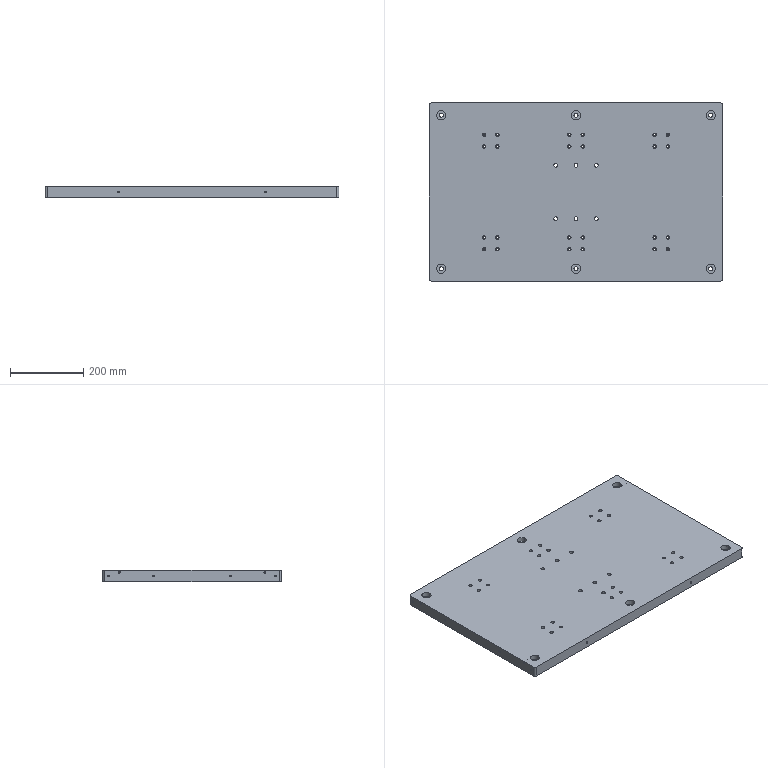NC program | Mastercam | posted with a generic post | part box 800 x 485 x 30 mm
Lines 2148 to 3510 of 3510:
N1620 T7 M6
N1630 G0 G90 G17 G54 X-367. Y-209. A0. S3000 M3
N1640 G43 H7 Z50. M8
N1650 G98 G81 Z-.7 R1. F300.
N1660 X-312. Y-167.
N1670 X-218.
N1680 Y-73.
N1690 X-312.
N1700 Y73.
N1710 X-367. Y209.
N1720 X-312. Y167.
N1730 X-218.
N1740 Y73.
N1750 X-47.
N1760 Y167.
N1770 X0. Y209.
N1780 X47. Y167.
N1790 Y73.
N1800 Y-73.
N1810 X-47.
N1820 Y-167.
N1830 X0. Y-209.
N1840 X47. Y-167.
N1850 X218. Y-73.
N1860 Y-167.
N1870 X312.
N1880 X367. Y-209.
N1890 X312. Y-73.
N1900 Y73.
N1910 X218.
N1920 Y167.
N1930 X312.
N1940 X367. Y209.
N1950 G80
N1960 M5
N1970 G91 G0 G28 Z0. M9
N1980 A0.
N1990 M01
N2000 T1 M6
N2010 G0 G90 G17 G54 X-367. Y-209. A0. S800 M3
N2020 G43 H1 Z50. M8
N2030 G98 G83 Z-24.8 R1. Q2. F100.
N2040 X0.
N2050 X367.
N2060 Y209.
N2070 X0.
N2080 X-367.
N2090 G80
N2100 M5
N2110 G91 G0 G28 Z0. M9
N2120 A0.
N2130 M01
N2140 T14 M6
N2150 G0 G90 G17 G54 X-312. Y-167. A0. S800 M3
N2160 G43 H14 Z50. M8
N2170 G98 G83 Z-24.8 R1. Q2. F100.
N2180 X-218.
N2190 Y-73.
N2200 X-312.
N2210 Y73.
N2220 Y167.
N2230 X-218.
N2240 Y73.
N2250 X-47.
N2260 Y167.
N2270 X47.
N2280 Y73.
N2290 Y-73.
N2300 X-47.
N2310 Y-167.
N2320 X47.
N2330 X218.
N2340 X312.
N2350 Y-73.
N2360 X218.
N2370 Y73.
N2380 Y167.
N2390 X312.
N2400 Y73.
N2410 G80
N2420 M5
N2430 G91 G0 G28 Z0. M9
N2440 A0.
N2450 M01
N2460 T9 M6
N2470 G0 G90 G17 G54 X-361.55 Y208. A0. S6500 M3
N2480 G43 H9 Z50. M8
N2490 Z1.2
N2500 G1 Z.2 F600.
N2510 X-360.55 F3500.
N2520 G3 X-359.55 Y209. I0. J1.
N2530 X-367. Y216.45 Z-.05 I-7.45 J0.
N2540 X-374.45 Y209. Z-.3 I0. J-7.45
N2550 X-367. Y201.55 Z-.55 I7.45 J0.
N2560 X-359.55 Y209. Z-.8 I0. J7.45
N2570 X-367. Y216.45 Z-1.05 I-7.45 J0.
N2580 X-374.45 Y209. Z-1.3 I0. J-7.45
N2590 X-367. Y201.55 Z-1.55 I7.45 J0.
N2600 X-359.55 Y209. Z-1.8 I0. J7.45
N2610 X-367. Y216.45 Z-2.05 I-7.45 J0.
N2620 X-374.45 Y209. Z-2.3 I0. J-7.45
N2630 X-367. Y201.55 Z-2.55 I7.45 J0.
N2640 X-359.55 Y209. Z-2.8 I0. J7.45
N2650 X-367. Y216.45 Z-3.05 I-7.45 J0.
N2660 X-374.45 Y209. Z-3.3 I0. J-7.45
N2670 X-367. Y201.55 Z-3.55 I7.45 J0.
N2680 X-359.55 Y209. Z-3.8 I0. J7.45
N2690 X-367. Y216.45 Z-4.05 I-7.45 J0.
N2700 X-374.45 Y209. Z-4.3 I0. J-7.45
N2710 X-367. Y201.55 Z-4.55 I7.45 J0.
N2720 X-359.55 Y209. Z-4.8 I0. J7.45
N2730 X-367. Y216.45 Z-5.05 I-7.45 J0.
N2740 X-374.45 Y209. Z-5.3 I0. J-7.45
N2750 X-367. Y201.55 Z-5.55 I7.45 J0.
N2760 X-359.55 Y209. Z-5.8 I0. J7.45
N2770 X-367. Y216.45 Z-6.05 I-7.45 J0.
N2780 X-374.45 Y209. Z-6.3 I0. J-7.45
N2790 X-367. Y201.55 Z-6.55 I7.45 J0.
N2800 X-359.55 Y209. Z-6.8 I0. J7.45
N2810 X-367. Y216.45 Z-7.05 I-7.45 J0.
N2820 X-374.45 Y209. Z-7.3 I0. J-7.45
N2830 X-367. Y201.55 Z-7.55 I7.45 J0.
N2840 X-359.55 Y209. Z-7.8 I0. J7.45
N2850 X-367. Y216.45 Z-8.05 I-7.45 J0.
N2860 X-374.45 Y209. Z-8.3 I0. J-7.45
N2870 X-367. Y201.55 Z-8.55 I7.45 J0.
N2880 X-359.55 Y209. Z-8.8 I0. J7.45
N2890 X-367. Y216.45 Z-9.05 I-7.45 J0.
N2900 X-374.45 Y209. Z-9.3 I0. J-7.45
N2910 X-367. Y201.55 Z-9.55 I7.45 J0.
N2920 X-359.55 Y209. Z-9.8 I0. J7.45
N2930 X-367. Y216.45 Z-10.05 I-7.45 J0.
N2940 X-374.45 Y209. Z-10.3 I0. J-7.45
N2950 X-367. Y201.55 Z-10.55 I7.45 J0.
N2960 X-359.55 Y209. Z-10.8 I0. J7.45
N2970 X-367. Y216.45 Z-11.05 I-7.45 J0.
N2980 X-374.45 Y209. Z-11.3 I0. J-7.45
N2990 X-367. Y201.55 Z-11.55 I7.45 J0.
N3000 X-359.55 Y209. Z-11.8 I0. J7.45
N3010 X-367. Y216.45 Z-12.05 I-7.45 J0.
N3020 X-374.45 Y209. Z-12.3 I0. J-7.45
N3030 X-367. Y201.55 Z-12.55 I7.45 J0.
N3040 X-359.55 Y209. Z-12.8 I0. J7.45
N3050 X-362.621 Y215.027 Z-12.95 I-7.45 J0.
N3060 X-367. Y216.45 I-4.379 J-6.027
N3070 X-374.45 Y209. I0. J-7.45
N3080 X-367. Y201.55 I7.45 J0.
N3090 X-359.55 Y209. I0. J7.45
N3100 X-362.621 Y215.027 I-7.45 J0.
N3110 X-363.209 Y215.218 I-.588 J-.809
N3120 X-364.018 Y214.806 I0. J-1.
N3130 G1 X-364.606 Y213.997
N3140 G0 Z50.
N3150 X-361.55 Y-210.
N3160 Z1.2
N3170 G1 Z.2 F600.
N3180 X-360.55 F3500.
N3190 G3 X-359.55 Y-209. I0. J1.
N3200 X-367. Y-201.55 Z-.05 I-7.45 J0.
N3210 X-374.45 Y-209. Z-.3 I0. J-7.45
N3220 X-367. Y-216.45 Z-.55 I7.45 J0.
N3230 X-359.55 Y-209. Z-.8 I0. J7.45
N3240 X-367. Y-201.55 Z-1.05 I-7.45 J0.
N3250 X-374.45 Y-209. Z-1.3 I0. J-7.45
N3260 X-367. Y-216.45 Z-1.55 I7.45 J0.
N3270 X-359.55 Y-209. Z-1.8 I0. J7.45
N3280 X-367. Y-201.55 Z-2.05 I-7.45 J0.
N3290 X-374.45 Y-209. Z-2.3 I0. J-7.45
N3300 X-367. Y-216.45 Z-2.55 I7.45 J0.
N3310 X-359.55 Y-209. Z-2.8 I0. J7.45
N3320 X-367. Y-201.55 Z-3.05 I-7.45 J0.
N3330 X-374.45 Y-209. Z-3.3 I0. J-7.45
N3340 X-367. Y-216.45 Z-3.55 I7.45 J0.
N3350 X-359.55 Y-209. Z-3.8 I0. J7.45
N3360 X-367. Y-201.55 Z-4.05 I-7.45 J0.
N3370 X-374.45 Y-209. Z-4.3 I0. J-7.45
N3380 X-367. Y-216.45 Z-4.55 I7.45 J0.
N3390 X-359.55 Y-209. Z-4.8 I0. J7.45
N3400 X-367. Y-201.55 Z-5.05 I-7.45 J0.
N3410 X-374.45 Y-209. Z-5.3 I0. J-7.45
N3420 X-367. Y-216.45 Z-5.55 I7.45 J0.
N3430 X-359.55 Y-209. Z-5.8 I0. J7.45
N3440 X-367. Y-201.55 Z-6.05 I-7.45 J0.
N3450 X-374.45 Y-209. Z-6.3 I0. J-7.45
N3460 X-367. Y-216.45 Z-6.55 I7.45 J0.
N3470 X-359.55 Y-209. Z-6.8 I0. J7.45
N3480 X-367. Y-201.55 Z-7.05 I-7.45 J0.
N3490 X-374.45 Y-209. Z-7.3 I0. J-7.45
N3500 X-367. Y-216.45 Z-7.55 I7.45 J0.
N3510 X-359.55 Y-209. Z-7.8 I0. J7.45
N3520 X-367. Y-201.55 Z-8.05 I-7.45 J0.
N3530 X-374.45 Y-209. Z-8.3 I0. J-7.45
N3540 X-367. Y-216.45 Z-8.55 I7.45 J0.
N3550 X-359.55 Y-209. Z-8.8 I0. J7.45
N3560 X-367. Y-201.55 Z-9.05 I-7.45 J0.
N3570 X-374.45 Y-209. Z-9.3 I0. J-7.45
N3580 X-367. Y-216.45 Z-9.55 I7.45 J0.
N3590 X-359.55 Y-209. Z-9.8 I0. J7.45
N3600 X-367. Y-201.55 Z-10.05 I-7.45 J0.
N3610 X-374.45 Y-209. Z-10.3 I0. J-7.45
N3620 X-367. Y-216.45 Z-10.55 I7.45 J0.
N3630 X-359.55 Y-209. Z-10.8 I0. J7.45
N3640 X-367. Y-201.55 Z-11.05 I-7.45 J0.
N3650 X-374.45 Y-209. Z-11.3 I0. J-7.45
N3660 X-367. Y-216.45 Z-11.55 I7.45 J0.
N3670 X-359.55 Y-209. Z-11.8 I0. J7.45
N3680 X-367. Y-201.55 Z-12.05 I-7.45 J0.
N3690 X-374.45 Y-209. Z-12.3 I0. J-7.45
N3700 X-367. Y-216.45 Z-12.55 I7.45 J0.
N3710 X-359.55 Y-209. Z-12.8 I0. J7.45
N3720 X-362.621 Y-202.973 Z-12.95 I-7.45 J0.
N3730 X-367. Y-201.55 I-4.379 J-6.027
N3740 X-374.45 Y-209. I0. J-7.45
N3750 X-367. Y-216.45 I7.45 J0.
N3760 X-359.55 Y-209. I0. J7.45
N3770 X-362.621 Y-202.973 I-7.45 J0.
N3780 X-363.209 Y-202.782 I-.588 J-.809
N3790 X-364.018 Y-203.194 I0. J-1.
N3800 G1 X-364.606 Y-204.003
N3810 G0 Z50.
N3820 X5.45 Y-210.
N3830 Z1.2
N3840 G1 Z.2 F600.
N3850 X6.45 F3500.
N3860 G3 X7.45 Y-209. I0. J1.
N3870 X0. Y-201.55 Z-.05 I-7.45 J0.
N3880 X-7.45 Y-209. Z-.3 I0. J-7.45
N3890 X0. Y-216.45 Z-.55 I7.45 J0.
N3900 X7.45 Y-209. Z-.8 I0. J7.45
N3910 X0. Y-201.55 Z-1.05 I-7.45 J0.
N3920 X-7.45 Y-209. Z-1.3 I0. J-7.45
N3930 X0. Y-216.45 Z-1.55 I7.45 J0.
N3940 X7.45 Y-209. Z-1.8 I0. J7.45
N3950 X0. Y-201.55 Z-2.05 I-7.45 J0.
N3960 X-7.45 Y-209. Z-2.3 I0. J-7.45
N3970 X0. Y-216.45 Z-2.55 I7.45 J0.
N3980 X7.45 Y-209. Z-2.8 I0. J7.45
N3990 X0. Y-201.55 Z-3.05 I-7.45 J0.
N4000 X-7.45 Y-209. Z-3.3 I0. J-7.45
N4010 X0. Y-216.45 Z-3.55 I7.45 J0.
N4020 X7.45 Y-209. Z-3.8 I0. J7.45
N4030 X0. Y-201.55 Z-4.05 I-7.45 J0.
N4040 X-7.45 Y-209. Z-4.3 I0. J-7.45
N4050 X0. Y-216.45 Z-4.55 I7.45 J0.
N4060 X7.45 Y-209. Z-4.8 I0. J7.45
N4070 X0. Y-201.55 Z-5.05 I-7.45 J0.
N4080 X-7.45 Y-209. Z-5.3 I0. J-7.45
N4090 X0. Y-216.45 Z-5.55 I7.45 J0.
N4100 X7.45 Y-209. Z-5.8 I0. J7.45
N4110 X0. Y-201.55 Z-6.05 I-7.45 J0.
N4120 X-7.45 Y-209. Z-6.3 I0. J-7.45
N4130 X0. Y-216.45 Z-6.55 I7.45 J0.
N4140 X7.45 Y-209. Z-6.8 I0. J7.45
N4150 X0. Y-201.55 Z-7.05 I-7.45 J0.
N4160 X-7.45 Y-209. Z-7.3 I0. J-7.45
N4170 X0. Y-216.45 Z-7.55 I7.45 J0.
N4180 X7.45 Y-209. Z-7.8 I0. J7.45
N4190 X0. Y-201.55 Z-8.05 I-7.45 J0.
N4200 X-7.45 Y-209. Z-8.3 I0. J-7.45
N4210 X0. Y-216.45 Z-8.55 I7.45 J0.
N4220 X7.45 Y-209. Z-8.8 I0. J7.45
N4230 X0. Y-201.55 Z-9.05 I-7.45 J0.
N4240 X-7.45 Y-209. Z-9.3 I0. J-7.45
N4250 X0. Y-216.45 Z-9.55 I7.45 J0.
N4260 X7.45 Y-209. Z-9.8 I0. J7.45
N4270 X0. Y-201.55 Z-10.05 I-7.45 J0.
N4280 X-7.45 Y-209. Z-10.3 I0. J-7.45
N4290 X0. Y-216.45 Z-10.55 I7.45 J0.
N4300 X7.45 Y-209. Z-10.8 I0. J7.45
N4310 X0. Y-201.55 Z-11.05 I-7.45 J0.
N4320 X-7.45 Y-209. Z-11.3 I0. J-7.45
N4330 X0. Y-216.45 Z-11.55 I7.45 J0.
N4340 X7.45 Y-209. Z-11.8 I0. J7.45
N4350 X0. Y-201.55 Z-12.05 I-7.45 J0.
N4360 X-7.45 Y-209. Z-12.3 I0. J-7.45
N4370 X0. Y-216.45 Z-12.55 I7.45 J0.
N4380 X7.45 Y-209. Z-12.8 I0. J7.45
N4390 X4.379 Y-202.973 Z-12.95 I-7.45 J0.
N4400 X0. Y-201.55 I-4.379 J-6.027
N4410 X-7.45 Y-209. I0. J-7.45
N4420 X0. Y-216.45 I7.45 J0.
N4430 X7.45 Y-209. I0. J7.45
N4440 X4.379 Y-202.973 I-7.45 J0.
N4450 X3.791 Y-202.782 I-.588 J-.809
N4460 X2.982 Y-203.194 I0. J-1.
N4470 G1 X2.394 Y-204.003
N4480 G0 Z50.
N4490 X372.45 Y-210.
N4500 Z1.2
N4510 G1 Z.2 F600.
N4520 X373.45 F3500.
N4530 G3 X374.45 Y-209. I0. J1.
N4540 X367. Y-201.55 Z-.05 I-7.45 J0.
N4550 X359.55 Y-209. Z-.3 I0. J-7.45
N4560 X367. Y-216.45 Z-.55 I7.45 J0.
N4570 X374.45 Y-209. Z-.8 I0. J7.45
N4580 X367. Y-201.55 Z-1.05 I-7.45 J0.
N4590 X359.55 Y-209. Z-1.3 I0. J-7.45
N4600 X367. Y-216.45 Z-1.55 I7.45 J0.
N4610 X374.45 Y-209. Z-1.8 I0. J7.45
N4620 X367. Y-201.55 Z-2.05 I-7.45 J0.
N4630 X359.55 Y-209. Z-2.3 I0. J-7.45
N4640 X367. Y-216.45 Z-2.55 I7.45 J0.
N4650 X374.45 Y-209. Z-2.8 I0. J7.45
N4660 X367. Y-201.55 Z-3.05 I-7.45 J0.
N4670 X359.55 Y-209. Z-3.3 I0. J-7.45
N4680 X367. Y-216.45 Z-3.55 I7.45 J0.
N4690 X374.45 Y-209. Z-3.8 I0. J7.45
N4700 X367. Y-201.55 Z-4.05 I-7.45 J0.
N4710 X359.55 Y-209. Z-4.3 I0. J-7.45
N4720 X367. Y-216.45 Z-4.55 I7.45 J0.
N4730 X374.45 Y-209. Z-4.8 I0. J7.45
N4740 X367. Y-201.55 Z-5.05 I-7.45 J0.
N4750 X359.55 Y-209. Z-5.3 I0. J-7.45
N4760 X367. Y-216.45 Z-5.55 I7.45 J0.
N4770 X374.45 Y-209. Z-5.8 I0. J7.45
N4780 X367. Y-201.55 Z-6.05 I-7.45 J0.
N4790 X359.55 Y-209. Z-6.3 I0. J-7.45
N4800 X367. Y-216.45 Z-6.55 I7.45 J0.
N4810 X374.45 Y-209. Z-6.8 I0. J7.45
N4820 X367. Y-201.55 Z-7.05 I-7.45 J0.
N4830 X359.55 Y-209. Z-7.3 I0. J-7.45
N4840 X367. Y-216.45 Z-7.55 I7.45 J0.
N4850 X374.45 Y-209. Z-7.8 I0. J7.45
N4860 X367. Y-201.55 Z-8.05 I-7.45 J0.
N4870 X359.55 Y-209. Z-8.3 I0. J-7.45
N4880 X367. Y-216.45 Z-8.55 I7.45 J0.
N4890 X374.45 Y-209. Z-8.8 I0. J7.45
N4900 X367. Y-201.55 Z-9.05 I-7.45 J0.
N4910 X359.55 Y-209. Z-9.3 I0. J-7.45
N4920 X367. Y-216.45 Z-9.55 I7.45 J0.
N4930 X374.45 Y-209. Z-9.8 I0. J7.45
N4940 X367. Y-201.55 Z-10.05 I-7.45 J0.
N4950 X359.55 Y-209. Z-10.3 I0. J-7.45
N4960 X367. Y-216.45 Z-10.55 I7.45 J0.
N4970 X374.45 Y-209. Z-10.8 I0. J7.45
N4980 X367. Y-201.55 Z-11.05 I-7.45 J0.
N4990 X359.55 Y-209. Z-11.3 I0. J-7.45
N5000 X367. Y-216.45 Z-11.55 I7.45 J0.
N5010 X374.45 Y-209. Z-11.8 I0. J7.45
N5020 X367. Y-201.55 Z-12.05 I-7.45 J0.
N5030 X359.55 Y-209. Z-12.3 I0. J-7.45
N5040 X367. Y-216.45 Z-12.55 I7.45 J0.
N5050 X374.45 Y-209. Z-12.8 I0. J7.45
N5060 X371.379 Y-202.973 Z-12.95 I-7.45 J0.
N5070 X367. Y-201.55 I-4.379 J-6.027
N5080 X359.55 Y-209. I0. J-7.45
N5090 X367. Y-216.45 I7.45 J0.
N5100 X374.45 Y-209. I0. J7.45
N5110 X371.379 Y-202.973 I-7.45 J0.
N5120 X370.791 Y-202.782 I-.588 J-.809
N5130 X369.982 Y-203.194 I0. J-1.
N5140 G1 X369.394 Y-204.003
N5150 G0 Z50.
N5160 X372.45 Y208.
N5170 Z1.2
N5180 G1 Z.2 F600.
N5190 X373.45 F3500.
N5200 G3 X374.45 Y209. I0. J1.
N5210 X367. Y216.45 Z-.05 I-7.45 J0.
N5220 X359.55 Y209. Z-.3 I0. J-7.45
N5230 X367. Y201.55 Z-.55 I7.45 J0.
N5240 X374.45 Y209. Z-.8 I0. J7.45
N5250 X367. Y216.45 Z-1.05 I-7.45 J0.
N5260 X359.55 Y209. Z-1.3 I0. J-7.45
N5270 X367. Y201.55 Z-1.55 I7.45 J0.
N5280 X374.45 Y209. Z-1.8 I0. J7.45
N5290 X367. Y216.45 Z-2.05 I-7.45 J0.
N5300 X359.55 Y209. Z-2.3 I0. J-7.45
N5310 X367. Y201.55 Z-2.55 I7.45 J0.
N5320 X374.45 Y209. Z-2.8 I0. J7.45
N5330 X367. Y216.45 Z-3.05 I-7.45 J0.
N5340 X359.55 Y209. Z-3.3 I0. J-7.45
N5350 X367. Y201.55 Z-3.55 I7.45 J0.
N5360 X374.45 Y209. Z-3.8 I0. J7.45
N5370 X367. Y216.45 Z-4.05 I-7.45 J0.
N5380 X359.55 Y209. Z-4.3 I0. J-7.45
N5390 X367. Y201.55 Z-4.55 I7.45 J0.
N5400 X374.45 Y209. Z-4.8 I0. J7.45
N5410 X367. Y216.45 Z-5.05 I-7.45 J0.
N5420 X359.55 Y209. Z-5.3 I0. J-7.45
N5430 X367. Y201.55 Z-5.55 I7.45 J0.
N5440 X374.45 Y209. Z-5.8 I0. J7.45
N5450 X367. Y216.45 Z-6.05 I-7.45 J0.
N5460 X359.55 Y209. Z-6.3 I0. J-7.45
N5470 X367. Y201.55 Z-6.55 I7.45 J0.
N5480 X374.45 Y209. Z-6.8 I0. J7.45
N5490 X367. Y216.45 Z-7.05 I-7.45 J0.
N5500 X359.55 Y209. Z-7.3 I0. J-7.45
N5510 X367. Y201.55 Z-7.55 I7.45 J0.
N5520 X374.45 Y209. Z-7.8 I0. J7.45
N5530 X367. Y216.45 Z-8.05 I-7.45 J0.
N5540 X359.55 Y209. Z-8.3 I0. J-7.45
N5550 X367. Y201.55 Z-8.55 I7.45 J0.
N5560 X374.45 Y209. Z-8.8 I0. J7.45
N5570 X367. Y216.45 Z-9.05 I-7.45 J0.
N5580 X359.55 Y209. Z-9.3 I0. J-7.45
N5590 X367. Y201.55 Z-9.55 I7.45 J0.
N5600 X374.45 Y209. Z-9.8 I0. J7.45
N5610 X367. Y216.45 Z-10.05 I-7.45 J0.
N5620 X359.55 Y209. Z-10.3 I0. J-7.45
N5630 X367. Y201.55 Z-10.55 I7.45 J0.
N5640 X374.45 Y209. Z-10.8 I0. J7.45
N5650 X367. Y216.45 Z-11.05 I-7.45 J0.
N5660 X359.55 Y209. Z-11.3 I0. J-7.45
N5670 X367. Y201.55 Z-11.55 I7.45 J0.
N5680 X374.45 Y209. Z-11.8 I0. J7.45
N5690 X367. Y216.45 Z-12.05 I-7.45 J0.
N5700 X359.55 Y209. Z-12.3 I0. J-7.45
N5710 X367. Y201.55 Z-12.55 I7.45 J0.
N5720 X374.45 Y209. Z-12.8 I0. J7.45
N5730 X371.379 Y215.027 Z-12.95 I-7.45 J0.
N5740 X367. Y216.45 I-4.379 J-6.027
N5750 X359.55 Y209. I0. J-7.45
N5760 X367. Y201.55 I7.45 J0.
N5770 X374.45 Y209. I0. J7.45
N5780 X371.379 Y215.027 I-7.45 J0.
N5790 X370.791 Y215.218 I-.588 J-.809
N5800 X369.982 Y214.806 I0. J-1.
N5810 G1 X369.394 Y213.997
N5820 G0 Z50.
N5830 X5.45 Y208.
N5840 Z1.2
N5850 G1 Z.2 F600.
N5860 X6.45 F3500.
N5870 G3 X7.45 Y209. I0. J1.
N5880 X0. Y216.45 Z-.05 I-7.45 J0.
N5890 X-7.45 Y209. Z-.3 I0. J-7.45
N5900 X0. Y201.55 Z-.55 I7.45 J0.
N5910 X7.45 Y209. Z-.8 I0. J7.45
N5920 X0. Y216.45 Z-1.05 I-7.45 J0.
N5930 X-7.45 Y209. Z-1.3 I0. J-7.45
N5940 X0. Y201.55 Z-1.55 I7.45 J0.
N5950 X7.45 Y209. Z-1.8 I0. J7.45
N5960 X0. Y216.45 Z-2.05 I-7.45 J0.
N5970 X-7.45 Y209. Z-2.3 I0. J-7.45
N5980 X0. Y201.55 Z-2.55 I7.45 J0.
N5990 X7.45 Y209. Z-2.8 I0. J7.45
N6000 X0. Y216.45 Z-3.05 I-7.45 J0.
N6010 X-7.45 Y209. Z-3.3 I0. J-7.45
N6020 X0. Y201.55 Z-3.55 I7.45 J0.
N6030 X7.45 Y209. Z-3.8 I0. J7.45
N6040 X0. Y216.45 Z-4.05 I-7.45 J0.
N6050 X-7.45 Y209. Z-4.3 I0. J-7.45
N6060 X0. Y201.55 Z-4.55 I7.45 J0.
N6070 X7.45 Y209. Z-4.8 I0. J7.45
N6080 X0. Y216.45 Z-5.05 I-7.45 J0.
N6090 X-7.45 Y209. Z-5.3 I0. J-7.45
N6100 X0. Y201.55 Z-5.55 I7.45 J0.
N6110 X7.45 Y209. Z-5.8 I0. J7.45
N6120 X0. Y216.45 Z-6.05 I-7.45 J0.
N6130 X-7.45 Y209. Z-6.3 I0. J-7.45
N6140 X0. Y201.55 Z-6.55 I7.45 J0.
N6150 X7.45 Y209. Z-6.8 I0. J7.45
N6160 X0. Y216.45 Z-7.05 I-7.45 J0.
N6170 X-7.45 Y209. Z-7.3 I0. J-7.45
N6180 X0. Y201.55 Z-7.55 I7.45 J0.
N6190 X7.45 Y209. Z-7.8 I0. J7.45
N6200 X0. Y216.45 Z-8.05 I-7.45 J0.
N6210 X-7.45 Y209. Z-8.3 I0. J-7.45
N6220 X0. Y201.55 Z-8.55 I7.45 J0.
N6230 X7.45 Y209. Z-8.8 I0. J7.45
N6240 X0. Y216.45 Z-9.05 I-7.45 J0.
N6250 X-7.45 Y209. Z-9.3 I0. J-7.45
N6260 X0. Y201.55 Z-9.55 I7.45 J0.
N6270 X7.45 Y209. Z-9.8 I0. J7.45
N6280 X0. Y216.45 Z-10.05 I-7.45 J0.
N6290 X-7.45 Y209. Z-10.3 I0. J-7.45
N6300 X0. Y201.55 Z-10.55 I7.45 J0.
N6310 X7.45 Y209. Z-10.8 I0. J7.45
N6320 X0. Y216.45 Z-11.05 I-7.45 J0.
N6330 X-7.45 Y209. Z-11.3 I0. J-7.45
N6340 X0. Y201.55 Z-11.55 I7.45 J0.
N6350 X7.45 Y209. Z-11.8 I0. J7.45
N6360 X0. Y216.45 Z-12.05 I-7.45 J0.
N6370 X-7.45 Y209. Z-12.3 I0. J-7.45
N6380 X0. Y201.55 Z-12.55 I7.45 J0.
N6390 X7.45 Y209. Z-12.8 I0. J7.45
N6400 X4.379 Y215.027 Z-12.95 I-7.45 J0.
N6410 X0. Y216.45 I-4.379 J-6.027
N6420 X-7.45 Y209. I0. J-7.45
N6430 X0. Y201.55 I7.45 J0.
N6440 X7.45 Y209. I0. J7.45
N6450 X4.379 Y215.027 I-7.45 J0.
N6460 X3.791 Y215.218 I-.588 J-.809
N6470 X2.982 Y214.806 I0. J-1.
N6480 G1 X2.394 Y213.997
N6490 G0 Z50.
N6500 M5
N6510 G91 G28 Z0. M9
N6520 A0.
N6530 M01
N6540 T10 M6
N6550 G0 G90 G17 G54 X-361.47 Y208. A0. S6500 M3
N6560 G43 H10 Z50. M8
N6570 Z-12.
N6580 G1 Z-13. F600.
N6590 X-360.47 F1000.
N6600 G3 X-359.47 Y209. I0. J1.
N6610 X-367. Y216.53 I-7.53 J0.
N6620 X-374.53 Y209. I0. J-7.53
N6630 X-367. Y201.47 I7.53 J0.
N6640 X-359.47 Y209. I0. J7.53
N6650 X-360.47 Y210. I-1. J0.
N6660 G1 X-361.47
N6670 Y208.
N6680 X-360.47
N6690 G3 X-359.47 Y209. I0. J1.
N6700 X-367. Y216.53 I-7.53 J0.
N6710 X-374.53 Y209. I0. J-7.53
N6720 X-367. Y201.47 I7.53 J0.
N6730 X-359.47 Y209. I0. J7.53
N6740 X-360.47 Y210. I-1. J0.
N6750 G1 X-361.47
N6760 G0 Z50.
N6770 Y-210.
N6780 Z-12.
N6790 G1 Z-13. F600.
N6800 X-360.47 F1000.
N6810 G3 X-359.47 Y-209. I0. J1.
N6820 X-367. Y-201.47 I-7.53 J0.
N6830 X-374.53 Y-209. I0. J-7.53
N6840 X-367. Y-216.53 I7.53 J0.
N6850 X-359.47 Y-209. I0. J7.53
N6860 X-360.47 Y-208. I-1. J0.
N6870 G1 X-361.47
N6880 Y-210.
N6890 X-360.47
N6900 G3 X-359.47 Y-209. I0. J1.
N6910 X-367. Y-201.47 I-7.53 J0.
N6920 X-374.53 Y-209. I0. J-7.53
N6930 X-367. Y-216.53 I7.53 J0.
N6940 X-359.47 Y-209. I0. J7.53
N6950 X-360.47 Y-208. I-1. J0.
N6960 G1 X-361.47
N6970 G0 Z50.
N6980 X5.53 Y-210.
N6990 Z-12.
N7000 G1 Z-13. F600.
N7010 X6.53 F1000.
N7020 G3 X7.53 Y-209. I0. J1.
N7030 X0. Y-201.47 I-7.53 J0.
N7040 X-7.53 Y-209. I0. J-7.53
N7050 X0. Y-216.53 I7.53 J0.
N7060 X7.53 Y-209. I0. J7.53
N7070 X6.53 Y-208. I-1. J0.
N7080 G1 X5.53
N7090 Y-210.
N7100 X6.53
N7110 G3 X7.53 Y-209. I0. J1.
N7120 X0. Y-201.47 I-7.53 J0.
N7130 X-7.53 Y-209. I0. J-7.53
N7140 X0. Y-216.53 I7.53 J0.
N7150 X7.53 Y-209. I0. J7.53
N7160 X6.53 Y-208. I-1. J0.
N7170 G1 X5.53
N7180 G0 Z50.
N7190 X372.53 Y-210.
N7200 Z-12.
N7210 G1 Z-13. F600.
N7220 X373.53 F1000.
N7230 G3 X374.53 Y-209. I0. J1.
N7240 X367. Y-201.47 I-7.53 J0.
N7250 X359.47 Y-209. I0. J-7.53
N7260 X367. Y-216.53 I7.53 J0.
N7270 X374.53 Y-209. I0. J7.53
N7280 X373.53 Y-208. I-1. J0.
N7290 G1 X372.53
N7300 Y-210.
N7310 X373.53
N7320 G3 X374.53 Y-209. I0. J1.
N7330 X367. Y-201.47 I-7.53 J0.
N7340 X359.47 Y-209. I0. J-7.53
N7350 X367. Y-216.53 I7.53 J0.
N7360 X374.53 Y-209. I0. J7.53
N7370 X373.53 Y-208. I-1. J0.
N7380 G1 X372.53
N7390 G0 Z50.
N7400 Y208.
N7410 Z-12.
N7420 G1 Z-13. F600.
N7430 X373.53 F1000.
N7440 G3 X374.53 Y209. I0. J1.
N7450 X367. Y216.53 I-7.53 J0.
N7460 X359.47 Y209. I0. J-7.53
N7470 X367. Y201.47 I7.53 J0.
N7480 X374.53 Y209. I0. J7.53
N7490 X373.53 Y210. I-1. J0.
N7500 G1 X372.53
N7510 Y208.
N7520 X373.53
N7530 G3 X374.53 Y209. I0. J1.
N7540 X367. Y216.53 I-7.53 J0.
N7550 X359.47 Y209. I0. J-7.53
N7560 X367. Y201.47 I7.53 J0.
N7570 X374.53 Y209. I0. J7.53
N7580 X373.53 Y210. I-1. J0.
N7590 G1 X372.53
N7600 G0 Z50.
N7610 X5.53 Y208.
N7620 Z-12.
N7630 G1 Z-13. F600.
N7640 X6.53 F1000.
N7650 G3 X7.53 Y209. I0. J1.
N7660 X0. Y216.53 I-7.53 J0.
N7670 X-7.53 Y209. I0. J-7.53
N7680 X0. Y201.47 I7.53 J0.
N7690 X7.53 Y209. I0. J7.53
N7700 X6.53 Y210. I-1. J0.
N7710 G1 X5.53
N7720 Y208.
N7730 X6.53
N7740 G3 X7.53 Y209. I0. J1.
N7750 X0. Y216.53 I-7.53 J0.
N7760 X-7.53 Y209. I0. J-7.53
N7770 X0. Y201.47 I7.53 J0.
N7780 X7.53 Y209. I0. J7.53
N7790 X6.53 Y210. I-1. J0.
N7800 G1 X5.53
N7810 G0 Z50.
N7820 X-243.99 Y119.
N7830 Z1.
N7840 G1 Z-24.95 F600.
N7850 X-242.99 F1000.
N7860 G3 X-241.99 Y120. I0. J1.
N7870 X-265. Y143.01 I-23.01 J0.
N7880 X-288.01 Y120. I0. J-23.01
N7890 X-265. Y96.99 I23.01 J0.
N7900 X-241.99 Y120. I0. J23.01
N7910 X-242.99 Y121. I-1. J0.
N7920 G1 X-243.99
N7930 Y119.
N7940 X-242.99
N7950 G3 X-241.99 Y120. I0. J1.
N7960 X-265. Y143.01 I-23.01 J0.
N7970 X-288.01 Y120. I0. J-23.01
N7980 X-265. Y96.99 I23.01 J0.
N7990 X-241.99 Y120. I0. J23.01
N8000 X-242.99 Y121. I-1. J0.
N8010 G1 X-243.99
N8020 G0 Z50.
N8030 Y-121.
N8040 Z1.
N8050 G1 Z-24.95 F600.
N8060 X-242.99 F1000.
N8070 G3 X-241.99 Y-120. I0. J1.
N8080 X-265. Y-96.99 I-23.01 J0.
N8090 X-288.01 Y-120. I0. J-23.01
N8100 X-265. Y-143.01 I23.01 J0.
N8110 X-241.99 Y-120. I0. J23.01
N8120 X-242.99 Y-119. I-1. J0.
N8130 G1 X-243.99
N8140 Y-121.
N8150 X-242.99
N8160 G3 X-241.99 Y-120. I0. J1.
N8170 X-265. Y-96.99 I-23.01 J0.
N8180 X-288.01 Y-120. I0. J-23.01
N8190 X-265. Y-143.01 I23.01 J0.
N8200 X-241.99 Y-120. I0. J23.01
N8210 X-242.99 Y-119. I-1. J0.
N8220 G1 X-243.99
N8230 G0 Z50.
N8240 X21.01 Y-121.
N8250 Z1.
N8260 G1 Z-24.95 F600.
N8270 X22.01 F1000.
N8280 G3 X23.01 Y-120. I0. J1.
N8290 X0. Y-96.99 I-23.01 J0.
N8300 X-23.01 Y-120. I0. J-23.01
N8310 X0. Y-143.01 I23.01 J0.
N8320 X23.01 Y-120. I0. J23.01
N8330 X22.01 Y-119. I-1. J0.
N8340 G1 X21.01
N8350 Y-121.
N8360 X22.01
N8370 G3 X23.01 Y-120. I0. J1.
N8380 X0. Y-96.99 I-23.01 J0.
N8390 X-23.01 Y-120. I0. J-23.01
N8400 X0. Y-143.01 I23.01 J0.
N8410 X23.01 Y-120. I0. J23.01
N8420 X22.01 Y-119. I-1. J0.
N8430 G1 X21.01
N8440 G0 Z50.
N8450 Y119.
N8460 Z1.
N8470 G1 Z-24.95 F600.
N8480 X22.01 F1000.
N8490 G3 X23.01 Y120. I0. J1.
N8500 X0. Y143.01 I-23.01 J0.
N8510 X-23.01 Y120. I0. J-23.01
N8520 X0. Y96.99 I23.01 J0.
N8530 X23.01 Y120. I0. J23.01
N8540 X22.01 Y121. I-1. J0.
N8550 G1 X21.01
N8560 Y119.
N8570 X22.01
N8580 G3 X23.01 Y120. I0. J1.
N8590 X0. Y143.01 I-23.01 J0.
N8600 X-23.01 Y120. I0. J-23.01
N8610 X0. Y96.99 I23.01 J0.
N8620 X23.01 Y120. I0. J23.01
N8630 X22.01 Y121. I-1. J0.
N8640 G1 X21.01
N8650 G0 Z50.
N8660 X286.01 Y119.
N8670 Z1.
N8680 G1 Z-24.95 F600.
N8690 X287.01 F1000.
N8700 G3 X288.01 Y120. I0. J1.
N8710 X265. Y143.01 I-23.01 J0.
N8720 X241.99 Y120. I0. J-23.01
N8730 X265. Y96.99 I23.01 J0.
N8740 X288.01 Y120. I0. J23.01
N8750 X287.01 Y121. I-1. J0.
N8760 G1 X286.01
N8770 Y119.
N8780 X287.01
N8790 G3 X288.01 Y120. I0. J1.
N8800 X265. Y143.01 I-23.01 J0.
N8810 X241.99 Y120. I0. J-23.01
N8820 X265. Y96.99 I23.01 J0.
N8830 X288.01 Y120. I0. J23.01
N8840 X287.01 Y121. I-1. J0.
N8850 G1 X286.01
N8860 G0 Z50.
N8870 Y-121.
N8880 Z1.
N8890 G1 Z-24.95 F600.
N8900 X287.01 F1000.
N8910 G3 X288.01 Y-120. I0. J1.
N8920 X265. Y-96.99 I-23.01 J0.
N8930 X241.99 Y-120. I0. J-23.01
N8940 X265. Y-143.01 I23.01 J0.
N8950 X288.01 Y-120. I0. J23.01
N8960 X287.01 Y-119. I-1. J0.
N8970 G1 X286.01
N8980 Y-121.
N8990 X287.01
N9000 G3 X288.01 Y-120. I0. J1.
N9010 X265. Y-96.99 I-23.01 J0.
N9020 X241.99 Y-120. I0. J-23.01
N9030 X265. Y-143.01 I23.01 J0.
N9040 X288.01 Y-120. I0. J23.01
N9050 X287.01 Y-119. I-1. J0.
N9060 G1 X286.01
N9070 G0 Z50.
N9080 M5
N9090 G91 G28 Z0. M9
N9100 A0.
N9110 M01
N9120 T7 M6
N9130 G0 G90 G17 G54 X-355.95 Y208.6 A0. S6000 M3
N9140 G43 H7 Z50. M8
N9150 Z1.
N9160 G1 Z-.8 F600.
N9170 X-355.55 F1000.
N9180 G3 X-355.15 Y209. I0. J.4
N9190 X-367. Y220.85 I-11.85 J0.
N9200 X-378.85 Y209. I0. J-11.85
N9210 X-367. Y197.15 I11.85 J0.
N9220 X-355.15 Y209. I0. J11.85
N9230 X-355.55 Y209.4 I-.4 J0.
N9240 G1 X-355.95
N9250 G0 Z50.
N9260 X11.05 Y208.6
N9270 Z1.
N9280 G1 Z-.8 F600.
N9290 X11.45 F1000.
N9300 G3 X11.85 Y209. I0. J.4
N9310 X0. Y220.85 I-11.85 J0.
N9320 X-11.85 Y209. I0. J-11.85
N9330 X0. Y197.15 I11.85 J0.
N9340 X11.85 Y209. I0. J11.85
N9350 X11.45 Y209.4 I-.4 J0.
N9360 G1 X11.05
N9370 G0 Z50.
N9380 Y-209.4
N9390 Z1.
N9400 G1 Z-.8 F600.
N9410 X11.45 F1000.
N9420 G3 X11.85 Y-209. I0. J.4
N9430 X0. Y-197.15 I-11.85 J0.
N9440 X-11.85 Y-209. I0. J-11.85
N9450 X0. Y-220.85 I11.85 J0.
N9460 X11.85 Y-209. I0. J11.85
N9470 X11.45 Y-208.6 I-.4 J0.
N9480 G1 X11.05
N9490 G0 Z50.
N9500 X378.05 Y-209.4
N9510 Z1.
N9520 G1 Z-.8 F600.
N9530 X378.45 F1000.
N9540 G3 X378.85 Y-209. I0. J.4
N9550 X367. Y-197.15 I-11.85 J0.
N9560 X355.15 Y-209. I0. J-11.85
N9570 X367. Y-220.85 I11.85 J0.
N9580 X378.85 Y-209. I0. J11.85
N9590 X378.45 Y-208.6 I-.4 J0.
N9600 G1 X378.05
N9610 G0 Z50.
N9620 Y208.6
N9630 Z1.
N9640 G1 Z-.8 F600.
N9650 X378.45 F1000.
N9660 G3 X378.85 Y209. I0. J.4
N9670 X367. Y220.85 I-11.85 J0.
N9680 X355.15 Y209. I0. J-11.85
N9690 X367. Y197.15 I11.85 J0.
N9700 X378.85 Y209. I0. J11.85
N9710 X378.45 Y209.4 I-.4 J0.
N9720 G1 X378.05
N9730 G0 Z50.
N9740 X-355.95 Y-209.4
N9750 Z1.
N9760 G1 Z-.8 F600.
N9770 X-355.55 F1000.
N9780 G3 X-355.15 Y-209. I0. J.4
N9790 X-367. Y-197.15 I-11.85 J0.
N9800 X-378.85 Y-209. I0. J-11.85
N9810 X-367. Y-220.85 I11.85 J0.
N9820 X-355.15 Y-209. I0. J11.85
N9830 X-355.55 Y-208.6 I-.4 J0.
N9840 G1 X-355.95
N9850 G0 Z50.
N9860 X291.55 Y-120.4
N9870 Z1.
N9880 G1 Z-.8 F600.
N9890 X291.95 F1000.
N9900 G3 X292.35 Y-120. I0. J.4
N9910 X265. Y-92.65 I-27.35 J0.
N9920 X237.65 Y-120. I0. J-27.35
N9930 X265. Y-147.35 I27.35 J0.
N9940 X292.35 Y-120. I0. J27.35
N9950 X291.95 Y-119.6 I-.4 J0.
N9960 G1 X291.55
N9970 G0 Z50.
N9980 X315.8 Y-167.4
N9990 Z1.
N100 G1 Z-.8 F600.
N110 X316.2 F1000.
N120 G3 X316.6 Y-167. I0. J.4
N130 X312. Y-162.4 I-4.6 J0.
N140 X307.4 Y-167. I0. J-4.6
N150 X312. Y-171.6 I4.6 J0.
N160 X316.6 Y-167. I0. J4.6
N170 X316.2 Y-166.6 I-.4 J0.
N180 G1 X315.8
N190 G0 Z50.
N200 X221.8 Y-167.4
N210 Z1.
N220 G1 Z-.8 F600.
N230 X222.2 F1000.
N240 G3 X222.6 Y-167. I0. J.4
N250 X218. Y-162.4 I-4.6 J0.
N260 X213.4 Y-167. I0. J-4.6
N270 X218. Y-171.6 I4.6 J0.
N280 X222.6 Y-167. I0. J4.6
N290 X222.2 Y-166.6 I-.4 J0.
N300 G1 X221.8
N310 G0 Z50.
N320 Y-73.4
N330 Z1.
N340 G1 Z-.8 F600.
N350 X222.2 F1000.
N360 G3 X222.6 Y-73. I0. J.4
N370 X218. Y-68.4 I-4.6 J0.
N380 X213.4 Y-73. I0. J-4.6
N390 X218. Y-77.6 I4.6 J0.
N400 X222.6 Y-73. I0. J4.6
N410 X222.2 Y-72.6 I-.4 J0.
N420 G1 X221.8
N430 G0 Z50.
N440 X315.8 Y-73.4
N450 Z1.
N460 G1 Z-.8 F600.
N470 X316.2 F1000.
N480 G3 X316.6 Y-73. I0. J.4
N490 X312. Y-68.4 I-4.6 J0.
N500 X307.4 Y-73. I0. J-4.6
N510 X312. Y-77.6 I4.6 J0.
N520 X316.6 Y-73. I0. J4.6
N530 X316.2 Y-72.6 I-.4 J0.
N540 G1 X315.8
N550 G0 Z50.
N560 X-238.45 Y-120.4
N570 Z1.
N580 G1 Z-.8 F600.
N590 X-238.05 F1000.
N600 G3 X-237.65 Y-120. I0. J.4
N610 X-265. Y-92.65 I-27.35 J0.
N620 X-292.35 Y-120. I0. J-27.35
N630 X-265. Y-147.35 I27.35 J0.
N640 X-237.65 Y-120. I0. J27.35
N650 X-238.05 Y-119.6 I-.4 J0.
N660 G1 X-238.45
N670 G0 Z50.
N680 X-308.2 Y-167.4
N690 Z1.
N700 G1 Z-.8 F600.
N710 X-307.8 F1000.
N720 G3 X-307.4 Y-167. I0. J.4
N730 X-312. Y-162.4 I-4.6 J0.
N740 X-316.6 Y-167. I0. J-4.6
N750 X-312. Y-171.6 I4.6 J0.
N760 X-307.4 Y-167. I0. J4.6
N770 X-307.8 Y-166.6 I-.4 J0.
N780 G1 X-308.2
N790 G0 Z50.
N800 Y-73.4
N810 Z1.
N820 G1 Z-.8 F600.
N830 X-307.8 F1000.
N840 G3 X-307.4 Y-73. I0. J.4
N850 X-312. Y-68.4 I-4.6 J0.
N860 X-316.6 Y-73. I0. J-4.6
N870 X-312. Y-77.6 I4.6 J0.
N880 X-307.4 Y-73. I0. J4.6
N890 X-307.8 Y-72.6 I-.4 J0.
N900 G1 X-308.2
N910 G0 Z50.
N920 X50.8 Y-73.4
N930 Z1.
N940 G1 Z-.8 F600.
N950 X51.2 F1000.
N960 G3 X51.6 Y-73. I0. J.4
N970 X47. Y-68.4 I-4.6 J0.
N980 X42.4 Y-73. I0. J-4.6
N990 X47. Y-77.6 I4.6 J0.
N1000 X51.6 Y-73. I0. J4.6
N1010 X51.2 Y-72.6 I-.4 J0.
N1020 G1 X50.8
N1030 G0 Z50.
N1040 X-43.2 Y-73.4
N1050 Z1.
N1060 G1 Z-.8 F600.
N1070 X-42.8 F1000.
N1080 G3 X-42.4 Y-73. I0. J.4
N1090 X-47. Y-68.4 I-4.6 J0.
N1100 X-51.6 Y-73. I0. J-4.6
N1110 X-47. Y-77.6 I4.6 J0.
N1120 X-42.4 Y-73. I0. J4.6
N1130 X-42.8 Y-72.6 I-.4 J0.
N1140 G1 X-43.2
N1150 G0 Z50.
N1160 X26.55 Y-120.4
N1170 Z1.
N1180 G1 Z-.8 F600.
N1190 X26.95 F1000.
N1200 G3 X27.35 Y-120. I0. J.4
N1210 X0. Y-92.65 I-27.35 J0.
N1220 X-27.35 Y-120. I0. J-27.35
N1230 X0. Y-147.35 I27.35 J0.
N1240 X27.35 Y-120. I0. J27.35
N1250 X26.95 Y-119.6 I-.4 J0.
N1260 G1 X26.55
N1270 G0 Z50.
N1280 X-43.2 Y-167.4
N1290 Z1.
N1300 G1 Z-.8 F600.
N1310 X-42.8 F1000.
N1320 G3 X-42.4 Y-167. I0. J.4
N1330 X-47. Y-162.4 I-4.6 J0.
N1340 X-51.6 Y-167. I0. J-4.6
N1350 X-47. Y-171.6 I4.6 J0.
N1360 X-42.4 Y-167. I0. J4.6
N1370 X-42.8 Y-166.6 I-.4 J0.
N1380 G1 X-43.2
N1390 G0 Z50.
N1400 X50.8 Y-167.4
N1410 Z1.
N1420 G1 Z-.8 F600.
N1430 X51.2 F1000.
N1440 G3 X51.6 Y-167. I0. J.4
N1450 X47. Y-162.4 I-4.6 J0.
N1460 X42.4 Y-167. I0. J-4.6
N1470 X47. Y-171.6 I4.6 J0.
N1480 X51.6 Y-167. I0. J4.6
N1490 X51.2 Y-166.6 I-.4 J0.
N1500 G1 X50.8
N1510 G0 Z50.
N1520 X-214.2 Y72.6
N1530 Z1.
N1540 G1 Z-.8 F600.
N1550 X-213.8 F1000.
N1560 G3 X-213.4 Y73. I0. J.4
N1570 X-218. Y77.6 I-4.6 J0.
N1580 X-222.6 Y73. I0. J-4.6
N1590 X-218. Y68.4 I4.6 J0.
N1600 X-213.4 Y73. I0. J4.6
N1610 X-213.8 Y73.4 I-.4 J0.
N1620 G1 X-214.2
N1630 G0 Z50.
N1640 X-43.2 Y166.6
N1650 Z1.
N1660 G1 Z-.8 F600.
N1670 X-42.8 F1000.
N1680 G3 X-42.4 Y167. I0. J.4
N1690 X-47. Y171.6 I-4.6 J0.
N1700 X-51.6 Y167. I0. J-4.6
N1710 X-47. Y162.4 I4.6 J0.
N1720 X-42.4 Y167. I0. J4.6
N1730 X-42.8 Y167.4 I-.4 J0.
N1740 G1 X-43.2
N1750 G0 Z50.
N1760 Y72.6
N1770 Z1.
N1780 G1 Z-.8 F600.
N1790 X-42.8 F1000.
N1800 G3 X-42.4 Y73. I0. J.4
N1810 X-47. Y77.6 I-4.6 J0.
N1820 X-51.6 Y73. I0. J-4.6
N1830 X-47. Y68.4 I4.6 J0.
N1840 X-42.4 Y73. I0. J4.6
N1850 X-42.8 Y73.4 I-.4 J0.
N1860 G1 X-43.2
N1870 G0 Z50.
N1880 X26.55 Y119.6
N1890 Z1.
N1900 G1 Z-.8 F600.
N1910 X26.95 F1000.
N1920 G3 X27.35 Y120. I0. J.4
N1930 X0. Y147.35 I-27.35 J0.
N1940 X-27.35 Y120. I0. J-27.35
N1950 X0. Y92.65 I27.35 J0.
N1960 X27.35 Y120. I0. J27.35
N1970 X26.95 Y120.4 I-.4 J0.
N1980 G1 X26.55
N1990 G0 Z50.
N2000 X-308.2 Y72.6
N2010 Z1.
N2020 G1 Z-.8 F600.
N2030 X-307.8 F1000.
N2040 G3 X-307.4 Y73. I0. J.4
N2050 X-312. Y77.6 I-4.6 J0.
N2060 X-316.6 Y73. I0. J-4.6
N2070 X-312. Y68.4 I4.6 J0.
N2080 X-307.4 Y73. I0. J4.6
N2090 X-307.8 Y73.4 I-.4 J0.
N2100 G1 X-308.2
N2110 G0 Z50.
N2120 X-238.45 Y119.6
N2130 Z1.
N2140 G1 Z-.8 F600.
N2150 X-238.05 F1000.
N2160 G3 X-237.65 Y120. I0. J.4
N2170 X-265. Y147.35 I-27.35 J0.
N2180 X-292.35 Y120. I0. J-27.35
N2190 X-265. Y92.65 I27.35 J0.
N2200 X-237.65 Y120. I0. J27.35
N2210 X-238.05 Y120.4 I-.4 J0.
N2220 G1 X-238.45
N2230 G0 Z50.
N2240 X-214.2 Y166.6
N2250 Z1.
N2260 G1 Z-.8 F600.
N2270 X-213.8 F1000.
N2280 G3 X-213.4 Y167. I0. J.4
N2290 X-218. Y171.6 I-4.6 J0.
N2300 X-222.6 Y167. I0. J-4.6
N2310 X-218. Y162.4 I4.6 J0.
N2320 X-213.4 Y167. I0. J4.6
N2330 X-213.8 Y167.4 I-.4 J0.
N2340 G1 X-214.2
N2350 G0 Z50.
N2360 X-308.2 Y166.6
N2370 Z1.
N2380 G1 Z-.8 F600.
N2390 X-307.8 F1000.
N2400 G3 X-307.4 Y167. I0. J.4
N2410 X-312. Y171.6 I-4.6 J0.
N2420 X-316.6 Y167. I0. J-4.6
N2430 X-312. Y162.4 I4.6 J0.
N2440 X-307.4 Y167. I0. J4.6
N2450 X-307.8 Y167.4 I-.4 J0.
N2460 G1 X-308.2
N2470 G0 Z50.
N2480 X291.55 Y119.6
N2490 Z1.
N2500 G1 Z-.8 F600.
N2510 X291.95 F1000.
N2520 G3 X292.35 Y120. I0. J.4
N2530 X265. Y147.35 I-27.35 J0.
N2540 X237.65 Y120. I0. J-27.35
N2550 X265. Y92.65 I27.35 J0.
N2560 X292.35 Y120. I0. J27.35
N2570 X291.95 Y120.4 I-.4 J0.
N2580 G1 X291.55
N2590 G0 Z50.
N2600 X315.8 Y166.6
N2610 Z1.
N2620 G1 Z-.8 F600.
N2630 X316.2 F1000.
N2640 G3 X316.6 Y167. I0. J.4
N2650 X312. Y171.6 I-4.6 J0.
N2660 X307.4 Y167. I0. J-4.6
N2670 X312. Y162.4 I4.6 J0.
N2680 X316.6 Y167. I0. J4.6
N2690 X316.2 Y167.4 I-.4 J0.
N2700 G1 X315.8
N2710 G0 Z50.
N2720 Y72.6
N2730 Z1.
N2740 G1 Z-.8 F600.
N2750 X316.2 F1000.
N2760 G3 X316.6 Y73. I0. J.4
N2770 X312. Y77.6 I-4.6 J0.
N2780 X307.4 Y73. I0. J-4.6
N2790 X312. Y68.4 I4.6 J0.
N2800 X316.6 Y73. I0. J4.6
N2810 X316.2 Y73.4 I-.4 J0.
N2820 G1 X315.8
N2830 G0 Z50.
N2840 X221.8 Y72.6
N2850 Z1.
N2860 G1 Z-.8 F600.
N2870 X222.2 F1000.
N2880 G3 X222.6 Y73. I0. J.4
N2890 X218. Y77.6 I-4.6 J0.
N2900 X213.4 Y73. I0. J-4.6
N2910 X218. Y68.4 I4.6 J0.
N2920 X222.6 Y73. I0. J4.6
N2930 X222.2 Y73.4 I-.4 J0.
N2940 G1 X221.8
N2950 G0 Z50.
N2960 X50.8 Y72.6
N2970 Z1.
N2980 G1 Z-.8 F600.
N2990 X51.2 F1000.
N3000 G3 X51.6 Y73. I0. J.4
N3010 X47. Y77.6 I-4.6 J0.
N3020 X42.4 Y73. I0. J-4.6
N3030 X47. Y68.4 I4.6 J0.
N3040 X51.6 Y73. I0. J4.6
N3050 X51.2 Y73.4 I-.4 J0.
N3060 G1 X50.8
N3070 G0 Z50.
N3080 Y166.6
N3090 Z1.
N3100 G1 Z-.8 F600.
N3110 X51.2 F1000.
N3120 G3 X51.6 Y167. I0. J.4
N3130 X47. Y171.6 I-4.6 J0.
N3140 X42.4 Y167. I0. J-4.6
N3150 X47. Y162.4 I4.6 J0.
N3160 X51.6 Y167. I0. J4.6
N3170 X51.2 Y167.4 I-.4 J0.
N3180 G1 X50.8
N3190 G0 Z50.
N3200 X221.8 Y166.6
N3210 Z1.
N3220 G1 Z-.8 F600.
N3230 X222.2 F1000.
N3240 G3 X222.6 Y167. I0. J.4
N3250 X218. Y171.6 I-4.6 J0.
N3260 X213.4 Y167. I0. J-4.6
N3270 X218. Y162.4 I4.6 J0.
N3280 X222.6 Y167. I0. J4.6
N3290 X222.2 Y167.4 I-.4 J0.
N3300 G1 X221.8
N3310 G0 Z50.
N3320 X-214.2 Y-73.4
N3330 Z1.
N3340 G1 Z-.8 F600.
N3350 X-213.8 F1000.
N3360 G3 X-213.4 Y-73. I0. J.4
N3370 X-218. Y-68.4 I-4.6 J0.
N3380 X-222.6 Y-73. I0. J-4.6
N3390 X-218. Y-77.6 I4.6 J0.
N3400 X-213.4 Y-73. I0. J4.6
N3410 X-213.8 Y-72.6 I-.4 J0.
N3420 G1 X-214.2
N3430 G0 Z50.
N3440 Y-167.4
N3450 Z1.
N3460 G1 Z-.8 F600.
N3470 X-213.8 F1000.
N3480 G3 X-213.4 Y-167. I0. J.4
N3490 X-218. Y-162.4 I-4.6 J0.
N3500 X-222.6 Y-167. I0. J-4.6
N3510 X-218. Y-171.6 I4.6 J0.
N3520 X-213.4 Y-167. I0. J4.6
N3530 X-213.8 Y-166.6 I-.4 J0.
N3540 G1 X-214.2
N3550 G0 Z50.
N3560 X-362.95 Y208.6
N3570 Z-12.
N3580 G1 Z-13.8 F600.
N3590 X-362.55 F1000.
N3600 G3 X-362.15 Y209. I0. J.4
N3610 X-367. Y213.85 I-4.85 J0.
N3620 X-371.85 Y209. I0. J-4.85
N3630 X-367. Y204.15 I4.85 J0.
N3640 X-362.15 Y209. I0. J4.85
N3650 X-362.55 Y209.4 I-.4 J0.
N3660 G1 X-362.95
N3670 G0 Z50.
N3680 Y-209.4
N3690 Z-12.
N3700 G1 Z-13.8 F600.
N3710 X-362.55 F1000.
N3720 G3 X-362.15 Y-209. I0. J.4
N3730 X-367. Y-204.15 I-4.85 J0.
N3740 X-371.85 Y-209. I0. J-4.85
N3750 X-367. Y-213.85 I4.85 J0.
N3760 X-362.15 Y-209. I0. J4.85
N3770 X-362.55 Y-208.6 I-.4 J0.
N3780 G1 X-362.95
N3790 G0 Z50.
N3800 X4.05 Y-209.4
N3810 Z-12.
N3820 G1 Z-13.8 F600.
N3830 X4.45 F1000.
N3840 G3 X4.85 Y-209. I0. J.4
N3850 X0. Y-204.15 I-4.85 J0.
N3860 X-4.85 Y-209. I0. J-4.85
N3870 X0. Y-213.85 I4.85 J0.
N3880 X4.85 Y-209. I0. J4.85
N3890 X4.45 Y-208.6 I-.4 J0.
N3900 G1 X4.05
N3910 G0 Z50.
N3920 X371.05 Y-209.4
N3930 Z-12.
N3940 G1 Z-13.8 F600.
N3950 X371.45 F1000.
N3960 G3 X371.85 Y-209. I0. J.4
N3970 X367. Y-204.15 I-4.85 J0.
N3980 X362.15 Y-209. I0. J-4.85
N3990 X367. Y-213.85 I4.85 J0.
N4000 X371.85 Y-209. I0. J4.85
N4010 X371.45 Y-208.6 I-.4 J0.
N4020 G1 X371.05
N4030 G0 Z50.
N4040 Y208.6
N4050 Z-12.
N4060 G1 Z-13.8 F600.
N4070 X371.45 F1000.
N4080 G3 X371.85 Y209. I0. J.4
N4090 X367. Y213.85 I-4.85 J0.
N4100 X362.15 Y209. I0. J-4.85
N4110 X367. Y204.15 I4.85 J0.
N4120 X371.85 Y209. I0. J4.85
N4130 X371.45 Y209.4 I-.4 J0.
N4140 G1 X371.05
N4150 G0 Z50.
N4160 X4.05 Y208.6
N4170 Z-12.
N4180 G1 Z-13.8 F600.
N4190 X4.45 F1000.
N4200 G3 X4.85 Y209. I0. J.4
N4210 X0. Y213.85 I-4.85 J0.
N4220 X-4.85 Y209. I0. J-4.85
N4230 X0. Y204.15 I4.85 J0.
N4240 X4.85 Y209. I0. J4.85
N4250 X4.45 Y209.4 I-.4 J0.
N4260 G1 X4.05
N4270 G0 Z50.
N4280 X-200. Y0.
N4290 G98 G81 Z-.7 R1. F200.
N4300 X200.
N4310 G80
N4320 M5
N4330 G91 G0 G28 Z0. M9
N4340 A0.
N4350 M01
N4360 T18 M6
N4370 G0 G90 G17 G54 X-200. Y0. A0. S1200 M3
N4380 G43 H18 Z50. M8
N4390 G98 G83 Z-22. R1. Q2. F120.
N4400 X200.
N4410 G80
N4420 M5
N4430 G91 G0 G28 Z0. M9
N4440 A0.
N4450 M01
N4460 T7 M6
N4470 G0 G90 G17 G54 X-198.85 Y-.4 A0. S6000 M3
N4480 G43 H7 Z50. M8
N4490 Z1.
N4500 G1 Z-1. F600.
N4510 X-198.45 F1000.
N4520 G3 X-198.05 Y0. I0. J.4
N4530 X-200. Y1.95 I-1.95 J0.
N4540 X-201.95 Y0. I0. J-1.95
N4550 X-200. Y-1.95 I1.95 J0.
N4560 X-198.05 Y0. I0. J1.95
N4570 X-198.45 Y.4 I-.4 J0.
N4580 G1 X-198.85
N4590 G0 Z50.
N4600 X201.15 Y-.4
N4610 Z1.
N4620 G1 Z-1. F600.
N4630 X201.55 F1000.
N4640 G3 X201.95 Y0. I0. J.4
N4650 X200. Y1.95 I-1.95 J0.
N4660 X198.05 Y0. I0. J-1.95
N4670 X200. Y-1.95 I1.95 J0.
N4680 X201.95 Y0. I0. J1.95
N4690 X201.55 Y.4 I-.4 J0.
N4700 G1 X201.15
N4710 G0 Z50.
N4720 X-227.5 Y0.
N4730 G98 G81 Z-.7 R1. F200.
N4740 X0.
N4750 X227.5
N4760 G80
N4770 M5
N4780 G91 G0 G28 Z0. M9
N4790 A0.
N4800 M01
N4810 T18 M6
N4820 G0 G90 G17 G54 X-227.5 Y0. A0. S1200 M3
N4830 G43 H18 Z50. M8
N4840 G98 G83 Z-22. R1. Q2. F120.
N4850 X0.
N4860 X227.5
N4870 G80
N4880 M5
N4890 G91 G0 G28 Z0. M9
N4900 A0.
N4910 M01
N4920 T7 M6
N4930 G0 G90 G17 G54 X-226.35 Y-.4 A0. S6000 M3
N4940 G43 H7 Z50. M8
N4950 Z1.
N4960 G1 Z-1. F600.
N4970 X-225.95 F1000.
N4980 G3 X-225.55 Y0. I0. J.4
N4990 X-227.5 Y1.95 I-1.95 J0.
N5000 X-229.45 Y0. I0. J-1.95
N5010 X-227.5 Y-1.95 I1.95 J0.
N5020 X-225.55 Y0. I0. J1.95
N5030 X-225.95 Y.4 I-.4 J0.
N5040 G1 X-226.35
N5050 G0 Z50.
N5060 X1.15 Y-.4
N5070 Z1.
N5080 G1 Z-1. F600.
N5090 X1.55 F1000.
N5100 G3 X1.95 Y0. I0. J.4
N5110 X0. Y1.95 I-1.95 J0.
N5120 X-1.95 Y0. I0. J-1.95
N5130 X0. Y-1.95 I1.95 J0.
N5140 X1.95 Y0. I0. J1.95
N5150 X1.55 Y.4 I-.4 J0.
N5160 G1 X1.15
N5170 G0 Z50.
N5180 X228.65 Y-.4
N5190 Z1.
N5200 G1 Z-1. F600.
N5210 X229.05 F1000.
N5220 G3 X229.45 Y0. I0. J.4
N5230 X227.5 Y1.95 I-1.95 J0.
N5240 X225.55 Y0. I0. J-1.95
N5250 X227.5 Y-1.95 I1.95 J0.
N5260 X229.45 Y0. I0. J1.95
N5270 X229.05 Y.4 I-.4 J0.
N5280 G1 X228.65
N5290 G0 Z50.
N5300 M5
N5310 G91 G28 Z0. M9
N5320 G28 X0. Y0. A0.
N5330 M30
%